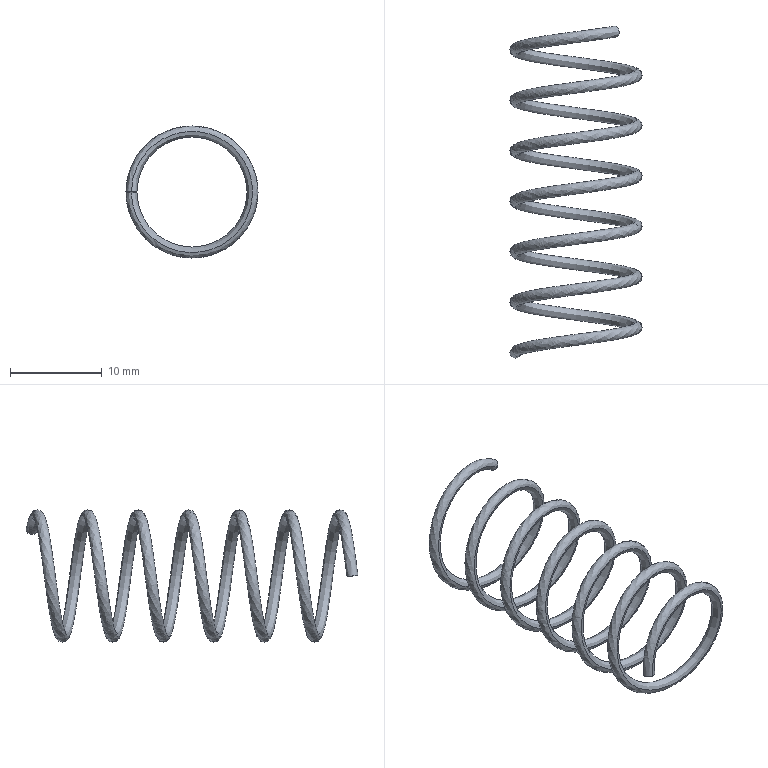Part | SolidWorks | features BaseBody 1 | 1 solid | 4 faces | volume 301.024 mm3 | spline 2 | plane 2